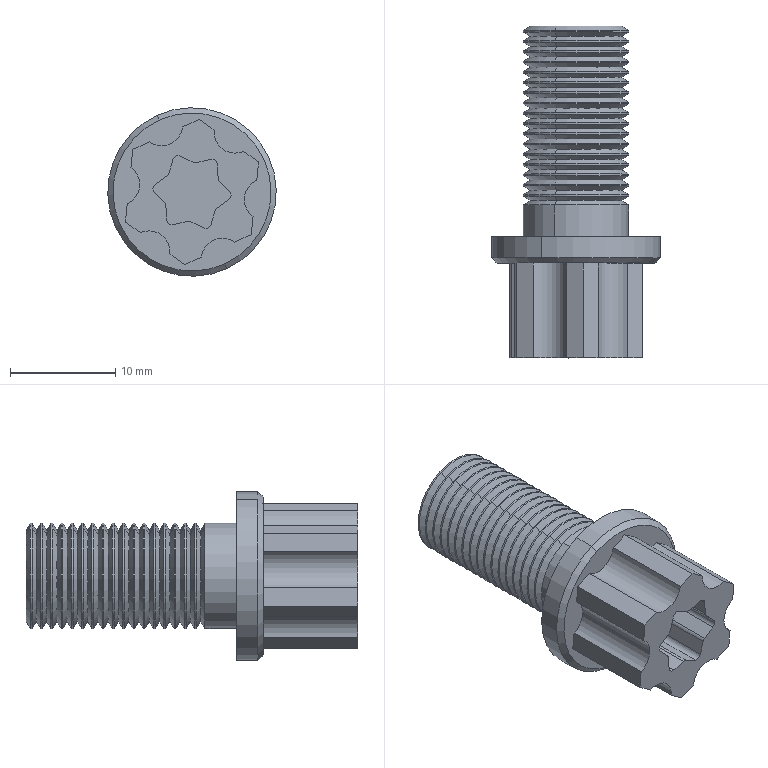Part | SolidWorks | features BaseBody 1 | 1 solid | 157 faces | box 16 x 31.5 x 16 mm | volume 2665 mm3 | cone 72 | cylinder 56 | plane 29 | commonest cylinder face diameters 10 x36 1 x12 4 x6 16 x2